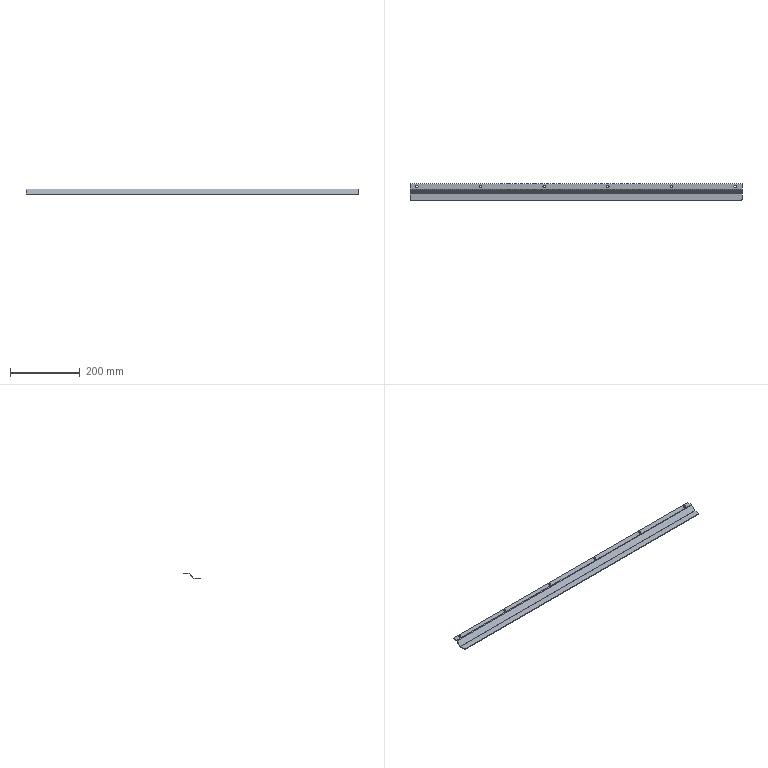Part | STEP file | 400v80 Rear Door Filler Piece | 1 solid | 28 faces | box 951 x 46.586 x 17 mm | volume 101104 mm3 | cylinder 18 | plane 10 | commonest cylinder face diameters 7 x12 1 x2 4 x2 5 x2
STEP:
#1=CARTESIAN_POINT('',(20.,15.239,-7.814));
#2=VERTEX_POINT('',#1);
#3=CARTESIAN_POINT('',(20.,22.239,-7.814));
#4=VERTEX_POINT('',#3);
#5=CARTESIAN_POINT('',(20.,18.739,-7.814));
#6=DIRECTION('',(0.,0.,-1.));
#7=DIRECTION('',(0.,1.,0.));
#8=AXIS2_PLACEMENT_3D('',#5,#6,#7);
#9=CIRCLE('',#8,3.5);
#10=EDGE_CURVE('',#2,#4,#9,.T.);
#11=ORIENTED_EDGE('',*,*,#10,.F.);
#12=CARTESIAN_POINT('',(20.,15.239,-9.814));
#13=VERTEX_POINT('',#12);
#14=CARTESIAN_POINT('',(20.,15.239,0.1865));
#15=DIRECTION('',(0.,0.,-1.));
#16=VECTOR('',#15,1000.);
#17=LINE('',#14,#16);
#18=EDGE_CURVE('',#2,#13,#17,.T.);
#19=ORIENTED_EDGE('',*,*,#18,.T.);
#20=CARTESIAN_POINT('',(20.,22.239,-9.814));
#21=VERTEX_POINT('',#20);
#22=CARTESIAN_POINT('',(20.,18.739,-9.814));
#23=DIRECTION('',(0.,0.,1.));
#24=DIRECTION('',(0.,1.,0.));
#25=AXIS2_PLACEMENT_3D('',#22,#23,#24);
#26=CIRCLE('',#25,3.5);
#27=EDGE_CURVE('',#21,#13,#26,.T.);
#28=ORIENTED_EDGE('',*,*,#27,.F.);
#29=CARTESIAN_POINT('',(20.,22.239,0.1865));
#30=DIRECTION('',(0.,0.,-1.));
#31=VECTOR('',#30,1000.);
#32=LINE('',#29,#31);
#33=EDGE_CURVE('',#4,#21,#32,.T.);
#34=ORIENTED_EDGE('',*,*,#33,.F.);
#35=EDGE_LOOP('',(#11,#19,#28,#34));
#36=FACE_OUTER_BOUND('',#35,.T.);
#37=CARTESIAN_POINT('',(20.,18.739,0.1865));
#38=DIRECTION('',(0.,0.,-1.));
#39=DIRECTION('',(0.,1.,0.));
#40=AXIS2_PLACEMENT_3D('',#37,#38,#39);
#41=CYLINDRICAL_SURFACE('',#40,3.5);
#42=ADVANCED_FACE('',(#36),#41,.F.);
#43=CARTESIAN_POINT('',(931.,15.239,-7.814));
#44=VERTEX_POINT('',#43);
#45=CARTESIAN_POINT('',(931.,22.239,-7.814));
#46=VERTEX_POINT('',#45);
#47=CARTESIAN_POINT('',(931.,18.739,-7.814));
#48=DIRECTION('',(0.,0.,-1.));
#49=DIRECTION('',(0.,1.,0.));
#50=AXIS2_PLACEMENT_3D('',#47,#48,#49);
#51=CIRCLE('',#50,3.5);
#52=EDGE_CURVE('',#44,#46,#51,.T.);
#53=ORIENTED_EDGE('',*,*,#52,.F.);
#54=CARTESIAN_POINT('',(931.,15.239,-9.814));
#55=VERTEX_POINT('',#54);
#56=CARTESIAN_POINT('',(931.,15.239,0.1865));
#57=DIRECTION('',(0.,0.,-1.));
#58=VECTOR('',#57,1000.);
#59=LINE('',#56,#58);
#60=EDGE_CURVE('',#44,#55,#59,.T.);
#61=ORIENTED_EDGE('',*,*,#60,.T.);
#62=CARTESIAN_POINT('',(931.,22.239,-9.814));
#63=VERTEX_POINT('',#62);
#64=CARTESIAN_POINT('',(931.,18.739,-9.814));
#65=DIRECTION('',(0.,0.,1.));
#66=DIRECTION('',(0.,1.,0.));
#67=AXIS2_PLACEMENT_3D('',#64,#65,#66);
#68=CIRCLE('',#67,3.5);
#69=EDGE_CURVE('',#63,#55,#68,.T.);
#70=ORIENTED_EDGE('',*,*,#69,.F.);
#71=CARTESIAN_POINT('',(931.,22.239,0.1865));
#72=DIRECTION('',(0.,0.,-1.));
#73=VECTOR('',#72,1000.);
#74=LINE('',#71,#73);
#75=EDGE_CURVE('',#46,#63,#74,.T.);
#76=ORIENTED_EDGE('',*,*,#75,.F.);
#77=EDGE_LOOP('',(#53,#61,#70,#76));
#78=FACE_OUTER_BOUND('',#77,.T.);
#79=CARTESIAN_POINT('',(931.,18.739,0.1865));
#80=DIRECTION('',(0.,0.,-1.));
#81=DIRECTION('',(0.,1.,0.));
#82=AXIS2_PLACEMENT_3D('',#79,#80,#81);
#83=CYLINDRICAL_SURFACE('',#82,3.5);
#84=ADVANCED_FACE('',(#78),#83,.F.);
#85=CARTESIAN_POINT('',(202.2,15.239,-7.814));
#86=VERTEX_POINT('',#85);
#87=CARTESIAN_POINT('',(202.2,22.239,-7.814));
#88=VERTEX_POINT('',#87);
#89=CARTESIAN_POINT('',(202.2,18.739,-7.814));
#90=DIRECTION('',(0.,0.,-1.));
#91=DIRECTION('',(0.,1.,0.));
#92=AXIS2_PLACEMENT_3D('',#89,#90,#91);
#93=CIRCLE('',#92,3.5);
#94=EDGE_CURVE('',#86,#88,#93,.T.);
#95=ORIENTED_EDGE('',*,*,#94,.F.);
#96=CARTESIAN_POINT('',(202.2,15.239,-9.814));
#97=VERTEX_POINT('',#96);
#98=CARTESIAN_POINT('',(202.2,15.239,0.1865));
#99=DIRECTION('',(0.,0.,-1.));
#100=VECTOR('',#99,1000.);
#101=LINE('',#98,#100);
#102=EDGE_CURVE('',#86,#97,#101,.T.);
#103=ORIENTED_EDGE('',*,*,#102,.T.);
#104=CARTESIAN_POINT('',(202.2,22.239,-9.814));
#105=VERTEX_POINT('',#104);
#106=CARTESIAN_POINT('',(202.2,18.739,-9.814));
#107=DIRECTION('',(0.,0.,1.));
#108=DIRECTION('',(0.,1.,0.));
#109=AXIS2_PLACEMENT_3D('',#106,#107,#108);
#110=CIRCLE('',#109,3.5);
#111=EDGE_CURVE('',#105,#97,#110,.T.);
#112=ORIENTED_EDGE('',*,*,#111,.F.);
#113=CARTESIAN_POINT('',(202.2,22.239,0.1865));
#114=DIRECTION('',(0.,0.,-1.));
#115=VECTOR('',#114,1000.);
#116=LINE('',#113,#115);
#117=EDGE_CURVE('',#88,#105,#116,.T.);
#118=ORIENTED_EDGE('',*,*,#117,.F.);
#119=EDGE_LOOP('',(#95,#103,#112,#118));
#120=FACE_OUTER_BOUND('',#119,.T.);
#121=CARTESIAN_POINT('',(202.2,18.739,0.1865));
#122=DIRECTION('',(0.,0.,-1.));
#123=DIRECTION('',(0.,1.,0.));
#124=AXIS2_PLACEMENT_3D('',#121,#122,#123);
#125=CYLINDRICAL_SURFACE('',#124,3.5);
#126=ADVANCED_FACE('',(#120),#125,.F.);
#127=CARTESIAN_POINT('',(384.4,15.239,-7.814));
#128=VERTEX_POINT('',#127);
#129=CARTESIAN_POINT('',(384.4,22.239,-7.814));
#130=VERTEX_POINT('',#129);
#131=CARTESIAN_POINT('',(384.4,18.739,-7.814));
#132=DIRECTION('',(0.,0.,-1.));
#133=DIRECTION('',(0.,1.,0.));
#134=AXIS2_PLACEMENT_3D('',#131,#132,#133);
#135=CIRCLE('',#134,3.5);
#136=EDGE_CURVE('',#128,#130,#135,.T.);
#137=ORIENTED_EDGE('',*,*,#136,.F.);
#138=CARTESIAN_POINT('',(384.4,15.239,-9.814));
#139=VERTEX_POINT('',#138);
#140=CARTESIAN_POINT('',(384.4,15.239,0.1865));
#141=DIRECTION('',(0.,0.,-1.));
#142=VECTOR('',#141,1000.);
#143=LINE('',#140,#142);
#144=EDGE_CURVE('',#128,#139,#143,.T.);
#145=ORIENTED_EDGE('',*,*,#144,.T.);
#146=CARTESIAN_POINT('',(384.4,22.239,-9.814));
#147=VERTEX_POINT('',#146);
#148=CARTESIAN_POINT('',(384.4,18.739,-9.814));
#149=DIRECTION('',(0.,0.,1.));
#150=DIRECTION('',(0.,1.,0.));
#151=AXIS2_PLACEMENT_3D('',#148,#149,#150);
#152=CIRCLE('',#151,3.5);
#153=EDGE_CURVE('',#147,#139,#152,.T.);
#154=ORIENTED_EDGE('',*,*,#153,.F.);
#155=CARTESIAN_POINT('',(384.4,22.239,0.1865));
#156=DIRECTION('',(0.,0.,-1.));
#157=VECTOR('',#156,1000.);
#158=LINE('',#155,#157);
#159=EDGE_CURVE('',#130,#147,#158,.T.);
#160=ORIENTED_EDGE('',*,*,#159,.F.);
#161=EDGE_LOOP('',(#137,#145,#154,#160));
#162=FACE_OUTER_BOUND('',#161,.T.);
#163=CARTESIAN_POINT('',(384.4,18.739,0.1865));
#164=DIRECTION('',(0.,0.,-1.));
#165=DIRECTION('',(0.,1.,0.));
#166=AXIS2_PLACEMENT_3D('',#163,#164,#165);
#167=CYLINDRICAL_SURFACE('',#166,3.5);
#168=ADVANCED_FACE('',(#162),#167,.F.);
#169=CARTESIAN_POINT('',(566.6,15.239,-7.814));
#170=VERTEX_POINT('',#169);
#171=CARTESIAN_POINT('',(566.6,22.239,-7.814));
#172=VERTEX_POINT('',#171);
#173=CARTESIAN_POINT('',(566.6,18.739,-7.814));
#174=DIRECTION('',(0.,0.,-1.));
#175=DIRECTION('',(0.,1.,0.));
#176=AXIS2_PLACEMENT_3D('',#173,#174,#175);
#177=CIRCLE('',#176,3.5);
#178=EDGE_CURVE('',#170,#172,#177,.T.);
#179=ORIENTED_EDGE('',*,*,#178,.F.);
#180=CARTESIAN_POINT('',(566.6,15.239,-9.814));
#181=VERTEX_POINT('',#180);
#182=CARTESIAN_POINT('',(566.6,15.239,0.1865));
#183=DIRECTION('',(0.,0.,-1.));
#184=VECTOR('',#183,1000.);
#185=LINE('',#182,#184);
#186=EDGE_CURVE('',#170,#181,#185,.T.);
#187=ORIENTED_EDGE('',*,*,#186,.T.);
#188=CARTESIAN_POINT('',(566.6,22.239,-9.814));
#189=VERTEX_POINT('',#188);
#190=CARTESIAN_POINT('',(566.6,18.739,-9.814));
#191=DIRECTION('',(0.,0.,1.));
#192=DIRECTION('',(0.,1.,0.));
#193=AXIS2_PLACEMENT_3D('',#190,#191,#192);
#194=CIRCLE('',#193,3.5);
#195=EDGE_CURVE('',#189,#181,#194,.T.);
#196=ORIENTED_EDGE('',*,*,#195,.F.);
#197=CARTESIAN_POINT('',(566.6,22.239,0.1865));
#198=DIRECTION('',(0.,0.,-1.));
#199=VECTOR('',#198,1000.);
#200=LINE('',#197,#199);
#201=EDGE_CURVE('',#172,#189,#200,.T.);
#202=ORIENTED_EDGE('',*,*,#201,.F.);
#203=EDGE_LOOP('',(#179,#187,#196,#202));
#204=FACE_OUTER_BOUND('',#203,.T.);
#205=CARTESIAN_POINT('',(566.6,18.739,0.1865));
#206=DIRECTION('',(0.,0.,-1.));
#207=DIRECTION('',(0.,1.,0.));
#208=AXIS2_PLACEMENT_3D('',#205,#206,#207);
#209=CYLINDRICAL_SURFACE('',#208,3.5);
#210=ADVANCED_FACE('',(#204),#209,.F.);
#211=CARTESIAN_POINT('',(748.8,15.239,-7.814));
#212=VERTEX_POINT('',#211);
#213=CARTESIAN_POINT('',(748.8,22.239,-7.814));
#214=VERTEX_POINT('',#213);
#215=CARTESIAN_POINT('',(748.8,18.739,-7.814));
#216=DIRECTION('',(0.,0.,-1.));
#217=DIRECTION('',(0.,1.,0.));
#218=AXIS2_PLACEMENT_3D('',#215,#216,#217);
#219=CIRCLE('',#218,3.5);
#220=EDGE_CURVE('',#212,#214,#219,.T.);
#221=ORIENTED_EDGE('',*,*,#220,.F.);
#222=CARTESIAN_POINT('',(748.8,15.239,-9.814));
#223=VERTEX_POINT('',#222);
#224=CARTESIAN_POINT('',(748.8,15.239,0.1865));
#225=DIRECTION('',(0.,0.,-1.));
#226=VECTOR('',#225,1000.);
#227=LINE('',#224,#226);
#228=EDGE_CURVE('',#212,#223,#227,.T.);
#229=ORIENTED_EDGE('',*,*,#228,.T.);
#230=CARTESIAN_POINT('',(748.8,22.239,-9.814));
#231=VERTEX_POINT('',#230);
#232=CARTESIAN_POINT('',(748.8,18.739,-9.814));
#233=DIRECTION('',(0.,0.,1.));
#234=DIRECTION('',(0.,1.,0.));
#235=AXIS2_PLACEMENT_3D('',#232,#233,#234);
#236=CIRCLE('',#235,3.5);
#237=EDGE_CURVE('',#231,#223,#236,.T.);
#238=ORIENTED_EDGE('',*,*,#237,.F.);
#239=CARTESIAN_POINT('',(748.8,22.239,0.1865));
#240=DIRECTION('',(0.,0.,-1.));
#241=VECTOR('',#240,1000.);
#242=LINE('',#239,#241);
#243=EDGE_CURVE('',#214,#231,#242,.T.);
#244=ORIENTED_EDGE('',*,*,#243,.F.);
#245=EDGE_LOOP('',(#221,#229,#238,#244));
#246=FACE_OUTER_BOUND('',#245,.T.);
#247=CARTESIAN_POINT('',(748.8,18.739,0.1865));
#248=DIRECTION('',(0.,0.,-1.));
#249=DIRECTION('',(0.,1.,0.));
#250=AXIS2_PLACEMENT_3D('',#247,#248,#249);
#251=CYLINDRICAL_SURFACE('',#250,3.5);
#252=ADVANCED_FACE('',(#246),#251,.F.);
#253=CARTESIAN_POINT('',(951.,10.972,-9.992));
#254=VERTEX_POINT('',#253);
#255=CARTESIAN_POINT('',(951.,-0.7152,-23.92));
#256=VERTEX_POINT('',#255);
#257=CARTESIAN_POINT('',(951.,11.122,-9.814));
#258=DIRECTION('',(0.,-0.6428,-0.766));
#259=VECTOR('',#258,1000.);
#260=LINE('',#257,#259);
#261=EDGE_CURVE('',#254,#256,#260,.T.);
#262=ORIENTED_EDGE('',*,*,#261,.T.);
#263=CARTESIAN_POINT('',(0.,-0.7152,-23.92));
#264=VERTEX_POINT('',#263);
#265=CARTESIAN_POINT('',(951.,-0.7152,-23.92));
#266=DIRECTION('',(-1.,0.,0.));
#267=VECTOR('',#266,1000.);
#268=LINE('',#265,#267);
#269=EDGE_CURVE('',#256,#264,#268,.T.);
#270=ORIENTED_EDGE('',*,*,#269,.T.);
#271=CARTESIAN_POINT('',(0.,10.972,-9.992));
#272=VERTEX_POINT('',#271);
#273=CARTESIAN_POINT('',(0.,11.122,-9.814));
#274=DIRECTION('',(0.,0.6428,0.766));
#275=VECTOR('',#274,1000.);
#276=LINE('',#273,#275);
#277=EDGE_CURVE('',#264,#272,#276,.T.);
#278=ORIENTED_EDGE('',*,*,#277,.T.);
#279=CARTESIAN_POINT('',(951.,10.972,-9.992));
#280=DIRECTION('',(1.,0.,0.));
#281=VECTOR('',#280,1000.);
#282=LINE('',#279,#281);
#283=EDGE_CURVE('',#272,#254,#282,.T.);
#284=ORIENTED_EDGE('',*,*,#283,.T.);
#285=EDGE_LOOP('',(#262,#270,#278,#284));
#286=FACE_OUTER_BOUND('',#285,.T.);
#287=CARTESIAN_POINT('',(951.,11.122,-9.814));
#288=DIRECTION('',(0.,0.766,-0.6428));
#289=DIRECTION('',(0.,0.6428,0.766));
#290=AXIS2_PLACEMENT_3D('',#287,#288,#289);
#291=PLANE('',#290);
#292=ADVANCED_FACE('',(#286),#291,.T.);
#293=CARTESIAN_POINT('',(951.,-2.63,-24.814));
#294=VERTEX_POINT('',#293);
#295=CARTESIAN_POINT('',(951.,-2.63,-22.314));
#296=DIRECTION('',(-1.,0.,0.));
#297=DIRECTION('',(0.,0.,1.));
#298=AXIS2_PLACEMENT_3D('',#295,#296,#297);
#299=CIRCLE('',#298,2.5);
#300=EDGE_CURVE('',#256,#294,#299,.T.);
#301=ORIENTED_EDGE('',*,*,#300,.T.);
#302=CARTESIAN_POINT('',(0.,-2.63,-24.814));
#303=VERTEX_POINT('',#302);
#304=CARTESIAN_POINT('',(951.,-2.63,-24.814));
#305=DIRECTION('',(-1.,0.,0.));
#306=VECTOR('',#305,1000.);
#307=LINE('',#304,#306);
#308=EDGE_CURVE('',#294,#303,#307,.T.);
#309=ORIENTED_EDGE('',*,*,#308,.T.);
#310=CARTESIAN_POINT('',(0.,-2.63,-22.314));
#311=DIRECTION('',(1.,0.,0.));
#312=DIRECTION('',(0.,0.,1.));
#313=AXIS2_PLACEMENT_3D('',#310,#311,#312);
#314=CIRCLE('',#313,2.5);
#315=EDGE_CURVE('',#303,#264,#314,.T.);
#316=ORIENTED_EDGE('',*,*,#315,.T.);
#317=ORIENTED_EDGE('',*,*,#269,.F.);
#318=EDGE_LOOP('',(#301,#309,#316,#317));
#319=FACE_OUTER_BOUND('',#318,.T.);
#320=CARTESIAN_POINT('',(951.,-2.63,-22.314));
#321=DIRECTION('',(-1.,0.,0.));
#322=DIRECTION('',(0.,0.,1.));
#323=AXIS2_PLACEMENT_3D('',#320,#321,#322);
#324=CYLINDRICAL_SURFACE('',#323,2.5);
#325=ADVANCED_FACE('',(#319),#324,.T.);
#326=CARTESIAN_POINT('',(951.,9.44,-8.707));
#327=VERTEX_POINT('',#326);
#328=CARTESIAN_POINT('',(951.,-2.247,-22.635));
#329=VERTEX_POINT('',#328);
#330=CARTESIAN_POINT('',(951.,9.44,-8.707));
#331=DIRECTION('',(0.,-0.6428,-0.766));
#332=VECTOR('',#331,1000.);
#333=LINE('',#330,#332);
#334=EDGE_CURVE('',#327,#329,#333,.T.);
#335=ORIENTED_EDGE('',*,*,#334,.T.);
#336=CARTESIAN_POINT('',(951.,-2.63,-22.814));
#337=VERTEX_POINT('',#336);
#338=CARTESIAN_POINT('',(951.,-2.63,-22.314));
#339=DIRECTION('',(-1.,0.,0.));
#340=DIRECTION('',(0.,0.,1.));
#341=AXIS2_PLACEMENT_3D('',#338,#339,#340);
#342=CIRCLE('',#341,0.5);
#343=EDGE_CURVE('',#329,#337,#342,.T.);
#344=ORIENTED_EDGE('',*,*,#343,.T.);
#345=CARTESIAN_POINT('',(951.,-18.465,-22.814));
#346=VERTEX_POINT('',#345);
#347=CARTESIAN_POINT('',(951.,-2.247,-22.814));
#348=DIRECTION('',(0.,-1.,0.));
#349=VECTOR('',#348,1000.);
#350=LINE('',#347,#349);
#351=EDGE_CURVE('',#337,#346,#350,.T.);
#352=ORIENTED_EDGE('',*,*,#351,.T.);
#353=CARTESIAN_POINT('',(951.,-18.465,-24.814));
#354=VERTEX_POINT('',#353);
#355=CARTESIAN_POINT('',(951.,-18.465,-24.814));
#356=DIRECTION('',(0.,0.,1.));
#357=VECTOR('',#356,1000.);
#358=LINE('',#355,#357);
#359=EDGE_CURVE('',#354,#346,#358,.T.);
#360=ORIENTED_EDGE('',*,*,#359,.F.);
#361=CARTESIAN_POINT('',(951.,-1.465,-24.814));
#362=DIRECTION('',(0.,-1.,0.));
#363=VECTOR('',#362,1000.);
#364=LINE('',#361,#363);
#365=EDGE_CURVE('',#294,#354,#364,.T.);
#366=ORIENTED_EDGE('',*,*,#365,.F.);
#367=ORIENTED_EDGE('',*,*,#300,.F.);
#368=ORIENTED_EDGE('',*,*,#261,.F.);
#369=CARTESIAN_POINT('',(951.,11.355,-9.814));
#370=VERTEX_POINT('',#369);
#371=CARTESIAN_POINT('',(951.,11.355,-10.314));
#372=DIRECTION('',(-1.,0.,0.));
#373=DIRECTION('',(0.,0.,1.));
#374=AXIS2_PLACEMENT_3D('',#371,#372,#373);
#375=CIRCLE('',#374,0.5);
#376=EDGE_CURVE('',#254,#370,#375,.T.);
#377=ORIENTED_EDGE('',*,*,#376,.T.);
#378=CARTESIAN_POINT('',(951.,26.122,-9.814));
#379=VERTEX_POINT('',#378);
#380=CARTESIAN_POINT('',(951.,26.122,-9.814));
#381=DIRECTION('',(0.,-1.,0.));
#382=VECTOR('',#381,1000.);
#383=LINE('',#380,#382);
#384=EDGE_CURVE('',#379,#370,#383,.T.);
#385=ORIENTED_EDGE('',*,*,#384,.F.);
#386=CARTESIAN_POINT('',(951.,26.122,-7.814));
#387=VERTEX_POINT('',#386);
#388=CARTESIAN_POINT('',(951.,26.122,-22.314));
#389=DIRECTION('',(0.,0.,1.));
#390=VECTOR('',#389,1000.);
#391=LINE('',#388,#390);
#392=EDGE_CURVE('',#379,#387,#391,.T.);
#393=ORIENTED_EDGE('',*,*,#392,.T.);
#394=CARTESIAN_POINT('',(951.,11.355,-7.814));
#395=VERTEX_POINT('',#394);
#396=CARTESIAN_POINT('',(951.,-2.63,-7.814));
#397=DIRECTION('',(0.,-1.,0.));
#398=VECTOR('',#397,1000.);
#399=LINE('',#396,#398);
#400=EDGE_CURVE('',#387,#395,#399,.T.);
#401=ORIENTED_EDGE('',*,*,#400,.T.);
#402=CARTESIAN_POINT('',(951.,11.355,-10.314));
#403=DIRECTION('',(1.,0.,0.));
#404=DIRECTION('',(0.,0.,1.));
#405=AXIS2_PLACEMENT_3D('',#402,#403,#404);
#406=CIRCLE('',#405,2.5);
#407=EDGE_CURVE('',#395,#327,#406,.T.);
#408=ORIENTED_EDGE('',*,*,#407,.T.);
#409=EDGE_LOOP('',(#335,#344,#352,#360,#366,#367,#368,#377,#385,#393,#401,#408));
#410=FACE_OUTER_BOUND('',#409,.T.);
#411=CARTESIAN_POINT('',(951.,11.355,-7.814));
#412=DIRECTION('',(1.,0.,0.));
#413=DIRECTION('',(0.,0.,-1.));
#414=AXIS2_PLACEMENT_3D('',#411,#412,#413);
#415=PLANE('',#414);
#416=ADVANCED_FACE('',(#410),#415,.T.);
#417=CARTESIAN_POINT('',(0.,11.355,-9.814));
#418=VERTEX_POINT('',#417);
#419=CARTESIAN_POINT('',(951.,11.355,-9.814));
#420=DIRECTION('',(-1.,0.,0.));
#421=VECTOR('',#420,1000.);
#422=LINE('',#419,#421);
#423=EDGE_CURVE('',#370,#418,#422,.T.);
#424=ORIENTED_EDGE('',*,*,#423,.F.);
#425=ORIENTED_EDGE('',*,*,#376,.F.);
#426=ORIENTED_EDGE('',*,*,#283,.F.);
#427=CARTESIAN_POINT('',(0.,11.355,-10.314));
#428=DIRECTION('',(1.,0.,0.));
#429=DIRECTION('',(0.,0.,1.));
#430=AXIS2_PLACEMENT_3D('',#427,#428,#429);
#431=CIRCLE('',#430,0.5);
#432=EDGE_CURVE('',#418,#272,#431,.T.);
#433=ORIENTED_EDGE('',*,*,#432,.F.);
#434=EDGE_LOOP('',(#424,#425,#426,#433));
#435=FACE_OUTER_BOUND('',#434,.T.);
#436=CARTESIAN_POINT('',(951.,11.355,-10.314));
#437=DIRECTION('',(-1.,0.,0.));
#438=DIRECTION('',(0.,0.,1.));
#439=AXIS2_PLACEMENT_3D('',#436,#437,#438);
#440=CYLINDRICAL_SURFACE('',#439,0.5);
#441=ADVANCED_FACE('',(#435),#440,.F.);
#442=CARTESIAN_POINT('',(0.,-2.247,-22.635));
#443=VERTEX_POINT('',#442);
#444=CARTESIAN_POINT('',(0.,9.44,-8.707));
#445=VERTEX_POINT('',#444);
#446=CARTESIAN_POINT('',(0.,-2.247,-22.635));
#447=DIRECTION('',(0.,0.6428,0.766));
#448=VECTOR('',#447,1000.);
#449=LINE('',#446,#448);
#450=EDGE_CURVE('',#443,#445,#449,.T.);
#451=ORIENTED_EDGE('',*,*,#450,.T.);
#452=CARTESIAN_POINT('',(0.,11.355,-7.814));
#453=VERTEX_POINT('',#452);
#454=CARTESIAN_POINT('',(0.,11.355,-10.314));
#455=DIRECTION('',(-1.,0.,0.));
#456=DIRECTION('',(0.,0.,1.));
#457=AXIS2_PLACEMENT_3D('',#454,#455,#456);
#458=CIRCLE('',#457,2.5);
#459=EDGE_CURVE('',#445,#453,#458,.T.);
#460=ORIENTED_EDGE('',*,*,#459,.T.);
#461=CARTESIAN_POINT('',(0.,26.122,-7.814));
#462=VERTEX_POINT('',#461);
#463=CARTESIAN_POINT('',(0.,9.44,-7.814));
#464=DIRECTION('',(0.,1.,0.));
#465=VECTOR('',#464,1000.);
#466=LINE('',#463,#465);
#467=EDGE_CURVE('',#453,#462,#466,.T.);
#468=ORIENTED_EDGE('',*,*,#467,.T.);
#469=CARTESIAN_POINT('',(0.,26.122,-9.814));
#470=VERTEX_POINT('',#469);
#471=CARTESIAN_POINT('',(0.,26.122,-7.814));
#472=DIRECTION('',(0.,0.,1.));
#473=VECTOR('',#472,1000.);
#474=LINE('',#471,#473);
#475=EDGE_CURVE('',#470,#462,#474,.T.);
#476=ORIENTED_EDGE('',*,*,#475,.F.);
#477=CARTESIAN_POINT('',(0.,26.122,-9.814));
#478=DIRECTION('',(0.,1.,0.));
#479=VECTOR('',#478,1000.);
#480=LINE('',#477,#479);
#481=EDGE_CURVE('',#418,#470,#480,.T.);
#482=ORIENTED_EDGE('',*,*,#481,.F.);
#483=ORIENTED_EDGE('',*,*,#432,.T.);
#484=ORIENTED_EDGE('',*,*,#277,.F.);
#485=ORIENTED_EDGE('',*,*,#315,.F.);
#486=CARTESIAN_POINT('',(0.,-18.465,-24.814));
#487=VERTEX_POINT('',#486);
#488=CARTESIAN_POINT('',(0.,-1.465,-24.814));
#489=DIRECTION('',(0.,1.,0.));
#490=VECTOR('',#489,1000.);
#491=LINE('',#488,#490);
#492=EDGE_CURVE('',#487,#303,#491,.T.);
#493=ORIENTED_EDGE('',*,*,#492,.F.);
#494=CARTESIAN_POINT('',(0.,-18.465,-22.814));
#495=VERTEX_POINT('',#494);
#496=CARTESIAN_POINT('',(0.,-18.465,-22.314));
#497=DIRECTION('',(0.,0.,-1.));
#498=VECTOR('',#497,1000.);
#499=LINE('',#496,#498);
#500=EDGE_CURVE('',#495,#487,#499,.T.);
#501=ORIENTED_EDGE('',*,*,#500,.F.);
#502=CARTESIAN_POINT('',(0.,-2.63,-22.814));
#503=VERTEX_POINT('',#502);
#504=CARTESIAN_POINT('',(0.,-2.63,-22.814));
#505=DIRECTION('',(0.,-1.,0.));
#506=VECTOR('',#505,1000.);
#507=LINE('',#504,#506);
#508=EDGE_CURVE('',#503,#495,#507,.T.);
#509=ORIENTED_EDGE('',*,*,#508,.F.);
#510=CARTESIAN_POINT('',(0.,-2.63,-22.314));
#511=DIRECTION('',(1.,0.,0.));
#512=DIRECTION('',(0.,0.,1.));
#513=AXIS2_PLACEMENT_3D('',#510,#511,#512);
#514=CIRCLE('',#513,0.5);
#515=EDGE_CURVE('',#503,#443,#514,.T.);
#516=ORIENTED_EDGE('',*,*,#515,.T.);
#517=EDGE_LOOP('',(#451,#460,#468,#476,#482,#483,#484,#485,#493,#501,#509,#516));
#518=FACE_OUTER_BOUND('',#517,.T.);
#519=CARTESIAN_POINT('',(0.,-2.63,-22.814));
#520=DIRECTION('',(-1.,0.,0.));
#521=DIRECTION('',(0.,0.,1.));
#522=AXIS2_PLACEMENT_3D('',#519,#520,#521);
#523=PLANE('',#522);
#524=ADVANCED_FACE('',(#518),#523,.T.);
#525=ORIENTED_EDGE('',*,*,#365,.T.);
#526=CARTESIAN_POINT('',(949.,-20.465,-24.814));
#527=VERTEX_POINT('',#526);
#528=CARTESIAN_POINT('',(949.,-18.465,-24.814));
#529=DIRECTION('',(0.,0.,-1.));
#530=DIRECTION('',(1.,0.,0.));
#531=AXIS2_PLACEMENT_3D('',#528,#529,#530);
#532=CIRCLE('',#531,2.);
#533=EDGE_CURVE('',#354,#527,#532,.T.);
#534=ORIENTED_EDGE('',*,*,#533,.T.);
#535=CARTESIAN_POINT('',(2.,-20.465,-24.814));
#536=VERTEX_POINT('',#535);
#537=CARTESIAN_POINT('',(951.,-20.465,-24.814));
#538=DIRECTION('',(-1.,0.,0.));
#539=VECTOR('',#538,1000.);
#540=LINE('',#537,#539);
#541=EDGE_CURVE('',#527,#536,#540,.T.);
#542=ORIENTED_EDGE('',*,*,#541,.T.);
#543=CARTESIAN_POINT('',(2.,-18.465,-24.814));
#544=DIRECTION('',(0.,0.,-1.));
#545=DIRECTION('',(-1.,0.,0.));
#546=AXIS2_PLACEMENT_3D('',#543,#544,#545);
#547=CIRCLE('',#546,2.);
#548=EDGE_CURVE('',#536,#487,#547,.T.);
#549=ORIENTED_EDGE('',*,*,#548,.T.);
#550=ORIENTED_EDGE('',*,*,#492,.T.);
#551=ORIENTED_EDGE('',*,*,#308,.F.);
#552=EDGE_LOOP('',(#525,#534,#542,#549,#550,#551));
#553=FACE_OUTER_BOUND('',#552,.T.);
#554=CARTESIAN_POINT('',(951.,-1.465,-24.814));
#555=DIRECTION('',(0.,0.,-1.));
#556=DIRECTION('',(0.,1.,0.));
#557=AXIS2_PLACEMENT_3D('',#554,#555,#556);
#558=PLANE('',#557);
#559=ADVANCED_FACE('',(#553),#558,.T.);
#560=CARTESIAN_POINT('',(951.,-2.247,-22.635));
#561=DIRECTION('',(-1.,0.,0.));
#562=VECTOR('',#561,1000.);
#563=LINE('',#560,#562);
#564=EDGE_CURVE('',#329,#443,#563,.T.);
#565=ORIENTED_EDGE('',*,*,#564,.F.);
#566=ORIENTED_EDGE('',*,*,#334,.F.);
#567=CARTESIAN_POINT('',(951.,9.44,-8.707));
#568=DIRECTION('',(1.,0.,0.));
#569=VECTOR('',#568,1000.);
#570=LINE('',#567,#569);
#571=EDGE_CURVE('',#445,#327,#570,.T.);
#572=ORIENTED_EDGE('',*,*,#571,.F.);
#573=ORIENTED_EDGE('',*,*,#450,.F.);
#574=EDGE_LOOP('',(#565,#566,#572,#573));
#575=FACE_OUTER_BOUND('',#574,.T.);
#576=CARTESIAN_POINT('',(951.,9.59,-8.528));
#577=DIRECTION('',(0.,0.766,-0.6428));
#578=DIRECTION('',(0.,0.6428,0.766));
#579=AXIS2_PLACEMENT_3D('',#576,#577,#578);
#580=PLANE('',#579);
#581=ADVANCED_FACE('',(#575),#580,.F.);
#582=ORIENTED_EDGE('',*,*,#384,.T.);
#583=ORIENTED_EDGE('',*,*,#423,.T.);
#584=ORIENTED_EDGE('',*,*,#481,.T.);
#585=CARTESIAN_POINT('',(951.,26.122,-9.814));
#586=DIRECTION('',(1.,0.,0.));
#587=VECTOR('',#586,1000.);
#588=LINE('',#585,#587);
#589=EDGE_CURVE('',#470,#379,#588,.T.);
#590=ORIENTED_EDGE('',*,*,#589,.T.);
#591=EDGE_LOOP('',(#582,#583,#584,#590));
#592=FACE_OUTER_BOUND('',#591,.T.);
#593=ORIENTED_EDGE('',*,*,#27,.T.);
#594=CARTESIAN_POINT('',(20.,18.739,-9.814));
#595=DIRECTION('',(0.,0.,1.));
#596=DIRECTION('',(0.,1.,0.));
#597=AXIS2_PLACEMENT_3D('',#594,#595,#596);
#598=CIRCLE('',#597,3.5);
#599=EDGE_CURVE('',#13,#21,#598,.T.);
#600=ORIENTED_EDGE('',*,*,#599,.T.);
#601=EDGE_LOOP('',(#593,#600));
#602=FACE_BOUND('',#601,.T.);
#603=ORIENTED_EDGE('',*,*,#69,.T.);
#604=CARTESIAN_POINT('',(931.,18.739,-9.814));
#605=DIRECTION('',(0.,0.,1.));
#606=DIRECTION('',(0.,1.,0.));
#607=AXIS2_PLACEMENT_3D('',#604,#605,#606);
#608=CIRCLE('',#607,3.5);
#609=EDGE_CURVE('',#55,#63,#608,.T.);
#610=ORIENTED_EDGE('',*,*,#609,.T.);
#611=EDGE_LOOP('',(#603,#610));
#612=FACE_BOUND('',#611,.T.);
#613=ORIENTED_EDGE('',*,*,#111,.T.);
#614=CARTESIAN_POINT('',(202.2,18.739,-9.814));
#615=DIRECTION('',(0.,0.,1.));
#616=DIRECTION('',(0.,1.,0.));
#617=AXIS2_PLACEMENT_3D('',#614,#615,#616);
#618=CIRCLE('',#617,3.5);
#619=EDGE_CURVE('',#97,#105,#618,.T.);
#620=ORIENTED_EDGE('',*,*,#619,.T.);
#621=EDGE_LOOP('',(#613,#620));
#622=FACE_BOUND('',#621,.T.);
#623=ORIENTED_EDGE('',*,*,#153,.T.);
#624=CARTESIAN_POINT('',(384.4,18.739,-9.814));
#625=DIRECTION('',(0.,0.,1.));
#626=DIRECTION('',(0.,1.,0.));
#627=AXIS2_PLACEMENT_3D('',#624,#625,#626);
#628=CIRCLE('',#627,3.5);
#629=EDGE_CURVE('',#139,#147,#628,.T.);
#630=ORIENTED_EDGE('',*,*,#629,.T.);
#631=EDGE_LOOP('',(#623,#630));
#632=FACE_BOUND('',#631,.T.);
#633=ORIENTED_EDGE('',*,*,#195,.T.);
#634=CARTESIAN_POINT('',(566.6,18.739,-9.814));
#635=DIRECTION('',(0.,0.,1.));
#636=DIRECTION('',(0.,1.,0.));
#637=AXIS2_PLACEMENT_3D('',#634,#635,#636);
#638=CIRCLE('',#637,3.5);
#639=EDGE_CURVE('',#181,#189,#638,.T.);
#640=ORIENTED_EDGE('',*,*,#639,.T.);
#641=EDGE_LOOP('',(#633,#640));
#642=FACE_BOUND('',#641,.T.);
#643=ORIENTED_EDGE('',*,*,#237,.T.);
#644=CARTESIAN_POINT('',(748.8,18.739,-9.814));
#645=DIRECTION('',(0.,0.,1.));
#646=DIRECTION('',(0.,1.,0.));
#647=AXIS2_PLACEMENT_3D('',#644,#645,#646);
#648=CIRCLE('',#647,3.5);
#649=EDGE_CURVE('',#223,#231,#648,.T.);
#650=ORIENTED_EDGE('',*,*,#649,.T.);
#651=EDGE_LOOP('',(#643,#650));
#652=FACE_BOUND('',#651,.T.);
#653=CARTESIAN_POINT('',(951.,26.122,-9.814));
#654=DIRECTION('',(0.,0.,-1.));
#655=DIRECTION('',(0.,1.,0.));
#656=AXIS2_PLACEMENT_3D('',#653,#654,#655);
#657=PLANE('',#656);
#658=ADVANCED_FACE('',(#592,#602,#612,#622,#632,#642,#652),#657,.T.);
#659=CARTESIAN_POINT('',(949.,-20.465,-22.814));
#660=VERTEX_POINT('',#659);
#661=CARTESIAN_POINT('',(949.,-18.465,-22.814));
#662=DIRECTION('',(0.,0.,-1.));
#663=DIRECTION('',(1.,0.,0.));
#664=AXIS2_PLACEMENT_3D('',#661,#662,#663);
#665=CIRCLE('',#664,2.);
#666=EDGE_CURVE('',#346,#660,#665,.T.);
#667=ORIENTED_EDGE('',*,*,#666,.T.);
#668=CARTESIAN_POINT('',(949.,-20.465,-24.814));
#669=DIRECTION('',(0.,0.,-1.));
#670=VECTOR('',#669,1000.);
#671=LINE('',#668,#670);
#672=EDGE_CURVE('',#660,#527,#671,.T.);
#673=ORIENTED_EDGE('',*,*,#672,.T.);
#674=ORIENTED_EDGE('',*,*,#533,.F.);
#675=ORIENTED_EDGE('',*,*,#359,.T.);
#676=EDGE_LOOP('',(#667,#673,#674,#675));
#677=FACE_OUTER_BOUND('',#676,.T.);
#678=CARTESIAN_POINT('',(949.,-18.465,-24.814));
#679=DIRECTION('',(0.,0.,1.));
#680=DIRECTION('',(1.,0.,0.));
#681=AXIS2_PLACEMENT_3D('',#678,#679,#680);
#682=CYLINDRICAL_SURFACE('',#681,2.);
#683=ADVANCED_FACE('',(#677),#682,.T.);
#684=CARTESIAN_POINT('',(2.,-20.465,-22.814));
#685=VERTEX_POINT('',#684);
#686=CARTESIAN_POINT('',(2.,-18.465,-22.814));
#687=DIRECTION('',(0.,0.,-1.));
#688=DIRECTION('',(-1.,0.,0.));
#689=AXIS2_PLACEMENT_3D('',#686,#687,#688);
#690=CIRCLE('',#689,2.);
#691=EDGE_CURVE('',#685,#495,#690,.T.);
#692=ORIENTED_EDGE('',*,*,#691,.T.);
#693=ORIENTED_EDGE('',*,*,#500,.T.);
#694=ORIENTED_EDGE('',*,*,#548,.F.);
#695=CARTESIAN_POINT('',(2.,-20.465,-22.314));
#696=DIRECTION('',(0.,0.,1.));
#697=VECTOR('',#696,1000.);
#698=LINE('',#695,#697);
#699=EDGE_CURVE('',#536,#685,#698,.T.);
#700=ORIENTED_EDGE('',*,*,#699,.T.);
#701=EDGE_LOOP('',(#692,#693,#694,#700));
#702=FACE_OUTER_BOUND('',#701,.T.);
#703=CARTESIAN_POINT('',(2.,-18.465,-22.314));
#704=DIRECTION('',(0.,0.,-1.));
#705=DIRECTION('',(-1.,0.,0.));
#706=AXIS2_PLACEMENT_3D('',#703,#704,#705);
#707=CYLINDRICAL_SURFACE('',#706,2.);
#708=ADVANCED_FACE('',(#702),#707,.T.);
#709=ORIENTED_EDGE('',*,*,#541,.F.);
#710=ORIENTED_EDGE('',*,*,#672,.F.);
#711=CARTESIAN_POINT('',(951.,-20.465,-22.814));
#712=DIRECTION('',(-1.,0.,0.));
#713=VECTOR('',#712,1000.);
#714=LINE('',#711,#713);
#715=EDGE_CURVE('',#660,#685,#714,.T.);
#716=ORIENTED_EDGE('',*,*,#715,.T.);
#717=ORIENTED_EDGE('',*,*,#699,.F.);
#718=EDGE_LOOP('',(#709,#710,#716,#717));
#719=FACE_OUTER_BOUND('',#718,.T.);
#720=CARTESIAN_POINT('',(951.,-20.465,-24.814));
#721=DIRECTION('',(0.,-1.,0.));
#722=DIRECTION('',(0.,0.,-1.));
#723=AXIS2_PLACEMENT_3D('',#720,#721,#722);
#724=PLANE('',#723);
#725=ADVANCED_FACE('',(#719),#724,.T.);
#726=CARTESIAN_POINT('',(951.,-2.63,-22.814));
#727=DIRECTION('',(-1.,0.,0.));
#728=VECTOR('',#727,1000.);
#729=LINE('',#726,#728);
#730=EDGE_CURVE('',#337,#503,#729,.T.);
#731=ORIENTED_EDGE('',*,*,#730,.F.);
#732=ORIENTED_EDGE('',*,*,#343,.F.);
#733=ORIENTED_EDGE('',*,*,#564,.T.);
#734=ORIENTED_EDGE('',*,*,#515,.F.);
#735=EDGE_LOOP('',(#731,#732,#733,#734));
#736=FACE_OUTER_BOUND('',#735,.T.);
#737=CARTESIAN_POINT('',(951.,-2.63,-22.314));
#738=DIRECTION('',(-1.,0.,0.));
#739=DIRECTION('',(0.,0.,1.));
#740=AXIS2_PLACEMENT_3D('',#737,#738,#739);
#741=CYLINDRICAL_SURFACE('',#740,0.5);
#742=ADVANCED_FACE('',(#736),#741,.F.);
#743=ORIENTED_EDGE('',*,*,#407,.F.);
#744=CARTESIAN_POINT('',(951.,11.355,-7.814));
#745=DIRECTION('',(-1.,0.,0.));
#746=VECTOR('',#745,1000.);
#747=LINE('',#744,#746);
#748=EDGE_CURVE('',#395,#453,#747,.T.);
#749=ORIENTED_EDGE('',*,*,#748,.T.);
#750=ORIENTED_EDGE('',*,*,#459,.F.);
#751=ORIENTED_EDGE('',*,*,#571,.T.);
#752=EDGE_LOOP('',(#743,#749,#750,#751));
#753=FACE_OUTER_BOUND('',#752,.T.);
#754=CARTESIAN_POINT('',(951.,11.355,-10.314));
#755=DIRECTION('',(-1.,0.,0.));
#756=DIRECTION('',(0.,0.,1.));
#757=AXIS2_PLACEMENT_3D('',#754,#755,#756);
#758=CYLINDRICAL_SURFACE('',#757,2.5);
#759=ADVANCED_FACE('',(#753),#758,.T.);
#760=ORIENTED_EDGE('',*,*,#392,.F.);
#761=ORIENTED_EDGE('',*,*,#589,.F.);
#762=ORIENTED_EDGE('',*,*,#475,.T.);
#763=CARTESIAN_POINT('',(951.,26.122,-7.814));
#764=DIRECTION('',(1.,0.,0.));
#765=VECTOR('',#764,1000.);
#766=LINE('',#763,#765);
#767=EDGE_CURVE('',#462,#387,#766,.T.);
#768=ORIENTED_EDGE('',*,*,#767,.T.);
#769=EDGE_LOOP('',(#760,#761,#762,#768));
#770=FACE_OUTER_BOUND('',#769,.T.);
#771=CARTESIAN_POINT('',(951.,26.122,-7.814));
#772=DIRECTION('',(0.,1.,0.));
#773=DIRECTION('',(0.,0.,1.));
#774=AXIS2_PLACEMENT_3D('',#771,#772,#773);
#775=PLANE('',#774);
#776=ADVANCED_FACE('',(#770),#775,.T.);
#777=ORIENTED_EDGE('',*,*,#18,.F.);
#778=CARTESIAN_POINT('',(20.,18.739,-7.814));
#779=DIRECTION('',(0.,0.,-1.));
#780=DIRECTION('',(0.,1.,0.));
#781=AXIS2_PLACEMENT_3D('',#778,#779,#780);
#782=CIRCLE('',#781,3.5);
#783=EDGE_CURVE('',#4,#2,#782,.T.);
#784=ORIENTED_EDGE('',*,*,#783,.F.);
#785=ORIENTED_EDGE('',*,*,#33,.T.);
#786=ORIENTED_EDGE('',*,*,#599,.F.);
#787=EDGE_LOOP('',(#777,#784,#785,#786));
#788=FACE_OUTER_BOUND('',#787,.T.);
#789=CARTESIAN_POINT('',(20.,18.739,0.1865));
#790=DIRECTION('',(0.,0.,-1.));
#791=DIRECTION('',(0.,1.,0.));
#792=AXIS2_PLACEMENT_3D('',#789,#790,#791);
#793=CYLINDRICAL_SURFACE('',#792,3.5);
#794=ADVANCED_FACE('',(#788),#793,.F.);
#795=ORIENTED_EDGE('',*,*,#60,.F.);
#796=CARTESIAN_POINT('',(931.,18.739,-7.814));
#797=DIRECTION('',(0.,0.,-1.));
#798=DIRECTION('',(0.,1.,0.));
#799=AXIS2_PLACEMENT_3D('',#796,#797,#798);
#800=CIRCLE('',#799,3.5);
#801=EDGE_CURVE('',#46,#44,#800,.T.);
#802=ORIENTED_EDGE('',*,*,#801,.F.);
#803=ORIENTED_EDGE('',*,*,#75,.T.);
#804=ORIENTED_EDGE('',*,*,#609,.F.);
#805=EDGE_LOOP('',(#795,#802,#803,#804));
#806=FACE_OUTER_BOUND('',#805,.T.);
#807=CARTESIAN_POINT('',(931.,18.739,0.1865));
#808=DIRECTION('',(0.,0.,-1.));
#809=DIRECTION('',(0.,1.,0.));
#810=AXIS2_PLACEMENT_3D('',#807,#808,#809);
#811=CYLINDRICAL_SURFACE('',#810,3.5);
#812=ADVANCED_FACE('',(#806),#811,.F.);
#813=ORIENTED_EDGE('',*,*,#102,.F.);
#814=CARTESIAN_POINT('',(202.2,18.739,-7.814));
#815=DIRECTION('',(0.,0.,-1.));
#816=DIRECTION('',(0.,1.,0.));
#817=AXIS2_PLACEMENT_3D('',#814,#815,#816);
#818=CIRCLE('',#817,3.5);
#819=EDGE_CURVE('',#88,#86,#818,.T.);
#820=ORIENTED_EDGE('',*,*,#819,.F.);
#821=ORIENTED_EDGE('',*,*,#117,.T.);
#822=ORIENTED_EDGE('',*,*,#619,.F.);
#823=EDGE_LOOP('',(#813,#820,#821,#822));
#824=FACE_OUTER_BOUND('',#823,.T.);
#825=CARTESIAN_POINT('',(202.2,18.739,0.1865));
#826=DIRECTION('',(0.,0.,-1.));
#827=DIRECTION('',(0.,1.,0.));
#828=AXIS2_PLACEMENT_3D('',#825,#826,#827);
#829=CYLINDRICAL_SURFACE('',#828,3.5);
#830=ADVANCED_FACE('',(#824),#829,.F.);
#831=ORIENTED_EDGE('',*,*,#144,.F.);
#832=CARTESIAN_POINT('',(384.4,18.739,-7.814));
#833=DIRECTION('',(0.,0.,-1.));
#834=DIRECTION('',(0.,1.,0.));
#835=AXIS2_PLACEMENT_3D('',#832,#833,#834);
#836=CIRCLE('',#835,3.5);
#837=EDGE_CURVE('',#130,#128,#836,.T.);
#838=ORIENTED_EDGE('',*,*,#837,.F.);
#839=ORIENTED_EDGE('',*,*,#159,.T.);
#840=ORIENTED_EDGE('',*,*,#629,.F.);
#841=EDGE_LOOP('',(#831,#838,#839,#840));
#842=FACE_OUTER_BOUND('',#841,.T.);
#843=CARTESIAN_POINT('',(384.4,18.739,0.1865));
#844=DIRECTION('',(0.,0.,-1.));
#845=DIRECTION('',(0.,1.,0.));
#846=AXIS2_PLACEMENT_3D('',#843,#844,#845);
#847=CYLINDRICAL_SURFACE('',#846,3.5);
#848=ADVANCED_FACE('',(#842),#847,.F.);
#849=ORIENTED_EDGE('',*,*,#186,.F.);
#850=CARTESIAN_POINT('',(566.6,18.739,-7.814));
#851=DIRECTION('',(0.,0.,-1.));
#852=DIRECTION('',(0.,1.,0.));
#853=AXIS2_PLACEMENT_3D('',#850,#851,#852);
#854=CIRCLE('',#853,3.5);
#855=EDGE_CURVE('',#172,#170,#854,.T.);
#856=ORIENTED_EDGE('',*,*,#855,.F.);
#857=ORIENTED_EDGE('',*,*,#201,.T.);
#858=ORIENTED_EDGE('',*,*,#639,.F.);
#859=EDGE_LOOP('',(#849,#856,#857,#858));
#860=FACE_OUTER_BOUND('',#859,.T.);
#861=CARTESIAN_POINT('',(566.6,18.739,0.1865));
#862=DIRECTION('',(0.,0.,-1.));
#863=DIRECTION('',(0.,1.,0.));
#864=AXIS2_PLACEMENT_3D('',#861,#862,#863);
#865=CYLINDRICAL_SURFACE('',#864,3.5);
#866=ADVANCED_FACE('',(#860),#865,.F.);
#867=ORIENTED_EDGE('',*,*,#228,.F.);
#868=CARTESIAN_POINT('',(748.8,18.739,-7.814));
#869=DIRECTION('',(0.,0.,-1.));
#870=DIRECTION('',(0.,1.,0.));
#871=AXIS2_PLACEMENT_3D('',#868,#869,#870);
#872=CIRCLE('',#871,3.5);
#873=EDGE_CURVE('',#214,#212,#872,.T.);
#874=ORIENTED_EDGE('',*,*,#873,.F.);
#875=ORIENTED_EDGE('',*,*,#243,.T.);
#876=ORIENTED_EDGE('',*,*,#649,.F.);
#877=EDGE_LOOP('',(#867,#874,#875,#876));
#878=FACE_OUTER_BOUND('',#877,.T.);
#879=CARTESIAN_POINT('',(748.8,18.739,0.1865));
#880=DIRECTION('',(0.,0.,-1.));
#881=DIRECTION('',(0.,1.,0.));
#882=AXIS2_PLACEMENT_3D('',#879,#880,#881);
#883=CYLINDRICAL_SURFACE('',#882,3.5);
#884=ADVANCED_FACE('',(#878),#883,.F.);
#885=ORIENTED_EDGE('',*,*,#691,.F.);
#886=ORIENTED_EDGE('',*,*,#715,.F.);
#887=ORIENTED_EDGE('',*,*,#666,.F.);
#888=ORIENTED_EDGE('',*,*,#351,.F.);
#889=ORIENTED_EDGE('',*,*,#730,.T.);
#890=ORIENTED_EDGE('',*,*,#508,.T.);
#891=EDGE_LOOP('',(#885,#886,#887,#888,#889,#890));
#892=FACE_OUTER_BOUND('',#891,.T.);
#893=CARTESIAN_POINT('',(951.,-1.465,-22.814));
#894=DIRECTION('',(0.,0.,-1.));
#895=DIRECTION('',(0.,1.,0.));
#896=AXIS2_PLACEMENT_3D('',#893,#894,#895);
#897=PLANE('',#896);
#898=ADVANCED_FACE('',(#892),#897,.F.);
#899=ORIENTED_EDGE('',*,*,#748,.F.);
#900=ORIENTED_EDGE('',*,*,#400,.F.);
#901=ORIENTED_EDGE('',*,*,#767,.F.);
#902=ORIENTED_EDGE('',*,*,#467,.F.);
#903=EDGE_LOOP('',(#899,#900,#901,#902));
#904=FACE_OUTER_BOUND('',#903,.T.);
#905=ORIENTED_EDGE('',*,*,#783,.T.);
#906=ORIENTED_EDGE('',*,*,#10,.T.);
#907=EDGE_LOOP('',(#905,#906));
#908=FACE_BOUND('',#907,.T.);
#909=ORIENTED_EDGE('',*,*,#801,.T.);
#910=ORIENTED_EDGE('',*,*,#52,.T.);
#911=EDGE_LOOP('',(#909,#910));
#912=FACE_BOUND('',#911,.T.);
#913=ORIENTED_EDGE('',*,*,#819,.T.);
#914=ORIENTED_EDGE('',*,*,#94,.T.);
#915=EDGE_LOOP('',(#913,#914));
#916=FACE_BOUND('',#915,.T.);
#917=ORIENTED_EDGE('',*,*,#837,.T.);
#918=ORIENTED_EDGE('',*,*,#136,.T.);
#919=EDGE_LOOP('',(#917,#918));
#920=FACE_BOUND('',#919,.T.);
#921=ORIENTED_EDGE('',*,*,#855,.T.);
#922=ORIENTED_EDGE('',*,*,#178,.T.);
#923=EDGE_LOOP('',(#921,#922));
#924=FACE_BOUND('',#923,.T.);
#925=ORIENTED_EDGE('',*,*,#873,.T.);
#926=ORIENTED_EDGE('',*,*,#220,.T.);
#927=EDGE_LOOP('',(#925,#926));
#928=FACE_BOUND('',#927,.T.);
#929=CARTESIAN_POINT('',(951.,26.122,-7.814));
#930=DIRECTION('',(0.,0.,-1.));
#931=DIRECTION('',(0.,1.,0.));
#932=AXIS2_PLACEMENT_3D('',#929,#930,#931);
#933=PLANE('',#932);
#934=ADVANCED_FACE('',(#904,#908,#912,#916,#920,#924,#928),#933,.F.);
#935=CLOSED_SHELL('',(#42,#84,#126,#168,#210,#252,#292,#325,#416,#441,#524,#559,#581,#658,#683,#708,#725,#742,#759,#776,#794,#812,#830,#848,#866,#884,#898,#934));
#936=MANIFOLD_SOLID_BREP('',#935);
#937=CARTESIAN_POINT('',(0.,0.,0.));
#938=DIRECTION('',(0.,0.,1.));
#939=DIRECTION('',(1.,0.,0.));
#940=AXIS2_PLACEMENT_3D('',#937,#938,#939);
#941=(LENGTH_UNIT()NAMED_UNIT(*)SI_UNIT(.MILLI.,.METRE.));
#942=UNCERTAINTY_MEASURE_WITH_UNIT(LENGTH_MEASURE(0.00001),#941,'','');
#943=(NAMED_UNIT(*)PLANE_ANGLE_UNIT()SI_UNIT($,.RADIAN.));
#944=(NAMED_UNIT(*)SI_UNIT($,.STERADIAN.)SOLID_ANGLE_UNIT());
#945=(GEOMETRIC_REPRESENTATION_CONTEXT(3)GLOBAL_UNCERTAINTY_ASSIGNED_CONTEXT((#942))GLOBAL_UNIT_ASSIGNED_CONTEXT((#941,#943,#944))REPRESENTATION_CONTEXT('',''));
#946=ADVANCED_BREP_SHAPE_REPRESENTATION('',(#936,#940),#945);